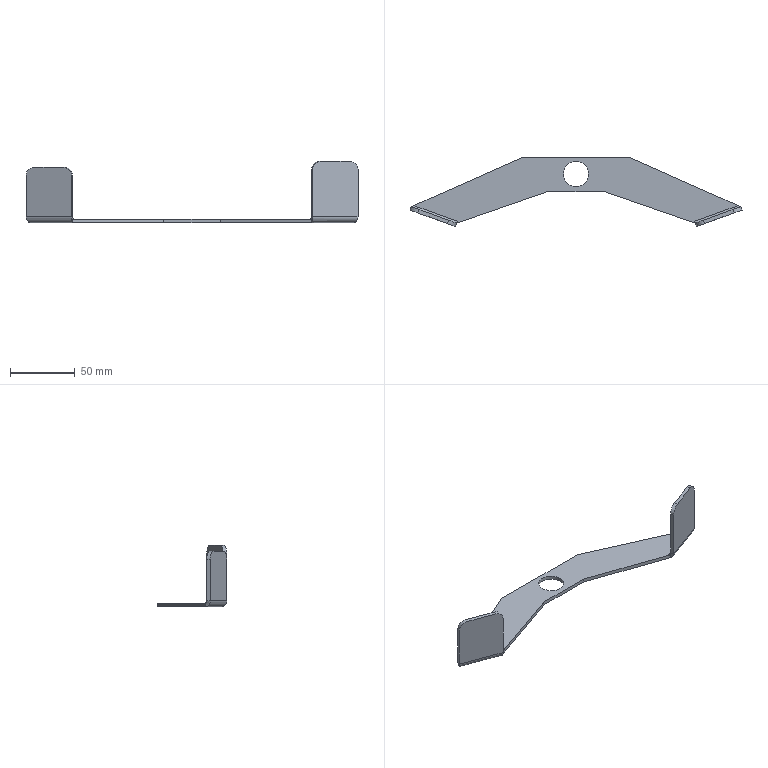Part | NX | features BREP 1 | 1 solid | 36 faces | box 255.894 x 53.402 x 47.219 mm | volume 25837 mm3 | plane 24 | cylinder 10 | spline 2 | commonest cylinder face diameters 12.7 x4 3.175 x2 8.712 x2 19.304 x2
STEP:
#1=CARTESIAN_POINT('',(124.91,13.64,0.));
#2=VERTEX_POINT('',#1);
#3=CARTESIAN_POINT('',(41.275,50.8,0.));
#4=VERTEX_POINT('',#3);
#5=CARTESIAN_POINT('',(124.91,13.64,0.));
#6=DIRECTION('',(-0.9139,0.406,0.));
#7=VECTOR('',#6,1000.);
#8=LINE('',#5,#7);
#9=EDGE_CURVE('',#2,#4,#8,.T.);
#10=ORIENTED_EDGE('',*,*,#9,.T.);
#11=CARTESIAN_POINT('',(-41.275,50.8,0.));
#12=VERTEX_POINT('',#11);
#13=CARTESIAN_POINT('',(41.275,50.8,0.));
#14=DIRECTION('',(-1.,0.,0.));
#15=VECTOR('',#14,1000.);
#16=LINE('',#13,#15);
#17=EDGE_CURVE('',#4,#12,#16,.T.);
#18=ORIENTED_EDGE('',*,*,#17,.T.);
#19=CARTESIAN_POINT('',(-124.91,13.64,0.));
#20=VERTEX_POINT('',#19);
#21=CARTESIAN_POINT('',(-41.275,50.8,0.));
#22=DIRECTION('',(-0.9139,-0.406,0.));
#23=VECTOR('',#22,1000.);
#24=LINE('',#21,#23);
#25=EDGE_CURVE('',#12,#20,#24,.T.);
#26=ORIENTED_EDGE('',*,*,#25,.T.);
#27=CARTESIAN_POINT('',(-91.532,1.492,0.));
#28=VERTEX_POINT('',#27);
#29=CARTESIAN_POINT('',(-124.91,13.64,0.));
#30=DIRECTION('',(0.9397,-0.342,0.));
#31=VECTOR('',#30,1000.);
#32=LINE('',#29,#31);
#33=EDGE_CURVE('',#20,#28,#32,.T.);
#34=ORIENTED_EDGE('',*,*,#33,.T.);
#35=CARTESIAN_POINT('',(-92.075,0.,0.));
#36=VERTEX_POINT('',#35);
#37=CARTESIAN_POINT('',(-91.532,1.492,0.));
#38=DIRECTION('',(-0.342,-0.9397,0.));
#39=VECTOR('',#38,1000.);
#40=LINE('',#37,#39);
#41=EDGE_CURVE('',#28,#36,#40,.T.);
#42=ORIENTED_EDGE('',*,*,#41,.T.);
#43=CARTESIAN_POINT('',(-21.717,24.384,0.));
#44=VERTEX_POINT('',#43);
#45=CARTESIAN_POINT('',(-92.075,0.,0.));
#46=DIRECTION('',(0.9449,0.3275,0.));
#47=VECTOR('',#46,1000.);
#48=LINE('',#45,#47);
#49=EDGE_CURVE('',#36,#44,#48,.T.);
#50=ORIENTED_EDGE('',*,*,#49,.T.);
#51=CARTESIAN_POINT('',(21.717,24.384,0.));
#52=VERTEX_POINT('',#51);
#53=CARTESIAN_POINT('',(-21.717,24.384,0.));
#54=DIRECTION('',(1.,0.,0.));
#55=VECTOR('',#54,1000.);
#56=LINE('',#53,#55);
#57=EDGE_CURVE('',#44,#52,#56,.T.);
#58=ORIENTED_EDGE('',*,*,#57,.T.);
#59=CARTESIAN_POINT('',(92.075,0.,0.));
#60=VERTEX_POINT('',#59);
#61=CARTESIAN_POINT('',(21.717,24.384,0.));
#62=DIRECTION('',(0.9449,-0.3275,0.));
#63=VECTOR('',#62,1000.);
#64=LINE('',#61,#63);
#65=EDGE_CURVE('',#52,#60,#64,.T.);
#66=ORIENTED_EDGE('',*,*,#65,.T.);
#67=CARTESIAN_POINT('',(91.532,1.492,0.));
#68=VERTEX_POINT('',#67);
#69=CARTESIAN_POINT('',(91.532,1.492,0.));
#70=DIRECTION('',(0.342,-0.9397,0.));
#71=VECTOR('',#70,1000.);
#72=LINE('',#69,#71);
#73=EDGE_CURVE('',#68,#60,#72,.T.);
#74=ORIENTED_EDGE('',*,*,#73,.F.);
#75=CARTESIAN_POINT('',(91.532,1.492,0.));
#76=DIRECTION('',(0.9397,0.342,0.));
#77=VECTOR('',#76,1000.);
#78=LINE('',#75,#77);
#79=EDGE_CURVE('',#68,#2,#78,.T.);
#80=ORIENTED_EDGE('',*,*,#79,.T.);
#81=EDGE_LOOP('',(#10,#18,#26,#34,#42,#50,#58,#66,#74,#80));
#82=FACE_BOUND('',#81,.T.);
#83=CARTESIAN_POINT('',(9.652,37.974,0.));
#84=VERTEX_POINT('',#83);
#85=CARTESIAN_POINT('',(-9.652,37.974,0.));
#86=VERTEX_POINT('',#85);
#87=CARTESIAN_POINT('',(0.,37.974,0.));
#88=DIRECTION('',(0.,0.,1.));
#89=DIRECTION('',(1.,0.,0.));
#90=AXIS2_PLACEMENT_3D('',#87,#88,#89);
#91=CIRCLE('',#90,9.652);
#92=EDGE_CURVE('',#84,#86,#91,.T.);
#93=ORIENTED_EDGE('',*,*,#92,.F.);
#94=CARTESIAN_POINT('',(0.,37.974,0.));
#95=DIRECTION('',(0.,0.,1.));
#96=DIRECTION('',(-1.,0.,0.));
#97=AXIS2_PLACEMENT_3D('',#94,#95,#96);
#98=CIRCLE('',#97,9.652);
#99=EDGE_CURVE('',#86,#84,#98,.T.);
#100=ORIENTED_EDGE('',*,*,#99,.F.);
#101=EDGE_LOOP('',(#93,#100));
#102=FACE_BOUND('',#101,.T.);
#103=CARTESIAN_POINT('',(0.,0.,0.));
#104=DIRECTION('',(0.,0.,1.));
#105=DIRECTION('',(1.,0.,0.));
#106=AXIS2_PLACEMENT_3D('',#103,#104,#105);
#107=PLANE('',#106);
#108=ADVANCED_FACE('',(#82,#102),#107,.T.);
#109=CARTESIAN_POINT('',(127.,12.712,1.587));
#110=VERTEX_POINT('',#109);
#111=CARTESIAN_POINT('',(127.,12.712,1.587));
#112=CARTESIAN_POINT('',(126.484,12.524,0.7563));
#113=CARTESIAN_POINT('',(125.71,13.047,0.));
#114=CARTESIAN_POINT('',(124.91,13.64,0.));
#115=B_SPLINE_CURVE_WITH_KNOTS('',3,(#111,#112,#113,#114),.UNSPECIFIED.,.F.,.F.,(4,4),(0.,1.),.UNSPECIFIED.);
#116=EDGE_CURVE('',#110,#2,#115,.T.);
#117=ORIENTED_EDGE('',*,*,#116,.T.);
#118=ORIENTED_EDGE('',*,*,#79,.F.);
#119=CARTESIAN_POINT('',(91.858,0.5973,0.3171));
#120=VERTEX_POINT('',#119);
#121=CARTESIAN_POINT('',(91.532,1.492,1.587));
#122=DIRECTION('',(0.9397,0.342,0.));
#123=DIRECTION('',(0.2051,-0.5635,-0.8003));
#124=AXIS2_PLACEMENT_3D('',#121,#122,#123);
#125=CIRCLE('',#124,1.587);
#126=EDGE_CURVE('',#120,#68,#125,.T.);
#127=ORIENTED_EDGE('',*,*,#126,.F.);
#128=CARTESIAN_POINT('',(92.075,0.,1.587));
#129=VERTEX_POINT('',#128);
#130=CARTESIAN_POINT('',(91.532,1.492,1.587));
#131=DIRECTION('',(0.9397,0.342,0.));
#132=DIRECTION('',(0.342,-0.9397,0.));
#133=AXIS2_PLACEMENT_3D('',#130,#131,#132);
#134=CIRCLE('',#133,1.587);
#135=EDGE_CURVE('',#129,#120,#134,.T.);
#136=ORIENTED_EDGE('',*,*,#135,.F.);
#137=CARTESIAN_POINT('',(92.075,0.,1.587));
#138=DIRECTION('',(0.9397,0.342,0.));
#139=VECTOR('',#138,1000.);
#140=LINE('',#137,#139);
#141=EDGE_CURVE('',#129,#110,#140,.T.);
#142=ORIENTED_EDGE('',*,*,#141,.T.);
#143=EDGE_LOOP('',(#117,#118,#127,#136,#142));
#144=FACE_BOUND('',#143,.T.);
#145=CARTESIAN_POINT('',(91.532,1.492,1.587));
#146=DIRECTION('',(0.9397,0.342,0.));
#147=DIRECTION('',(0.342,-0.9397,0.));
#148=AXIS2_PLACEMENT_3D('',#145,#146,#147);
#149=CYLINDRICAL_SURFACE('',#148,1.587);
#150=ADVANCED_FACE('',(#144),#149,.F.);
#151=ORIENTED_EDGE('',*,*,#141,.F.);
#152=CARTESIAN_POINT('',(92.075,0.,38.1));
#153=VERTEX_POINT('',#152);
#154=CARTESIAN_POINT('',(92.075,0.,38.1));
#155=DIRECTION('',(0.,0.,-1.));
#156=VECTOR('',#155,1000.);
#157=LINE('',#154,#156);
#158=EDGE_CURVE('',#153,#129,#157,.T.);
#159=ORIENTED_EDGE('',*,*,#158,.F.);
#160=CARTESIAN_POINT('',(98.042,2.172,44.45));
#161=VERTEX_POINT('',#160);
#162=CARTESIAN_POINT('',(98.042,2.172,38.1));
#163=DIRECTION('',(0.342,-0.9397,0.));
#164=DIRECTION('',(0.,0.,1.));
#165=AXIS2_PLACEMENT_3D('',#162,#163,#164);
#166=CIRCLE('',#165,6.35);
#167=EDGE_CURVE('',#161,#153,#166,.T.);
#168=ORIENTED_EDGE('',*,*,#167,.F.);
#169=CARTESIAN_POINT('',(121.033,10.54,44.45));
#170=VERTEX_POINT('',#169);
#171=CARTESIAN_POINT('',(121.033,10.54,44.45));
#172=DIRECTION('',(-0.9397,-0.342,0.));
#173=VECTOR('',#172,1000.);
#174=LINE('',#171,#173);
#175=EDGE_CURVE('',#170,#161,#174,.T.);
#176=ORIENTED_EDGE('',*,*,#175,.F.);
#177=CARTESIAN_POINT('',(127.,12.712,38.1));
#178=VERTEX_POINT('',#177);
#179=CARTESIAN_POINT('',(121.033,10.54,38.1));
#180=DIRECTION('',(0.342,-0.9397,0.));
#181=DIRECTION('',(0.9397,0.342,0.));
#182=AXIS2_PLACEMENT_3D('',#179,#180,#181);
#183=CIRCLE('',#182,6.35);
#184=EDGE_CURVE('',#178,#170,#183,.T.);
#185=ORIENTED_EDGE('',*,*,#184,.F.);
#186=CARTESIAN_POINT('',(127.,12.712,1.587));
#187=DIRECTION('',(0.,0.,1.));
#188=VECTOR('',#187,1000.);
#189=LINE('',#186,#188);
#190=EDGE_CURVE('',#110,#178,#189,.T.);
#191=ORIENTED_EDGE('',*,*,#190,.F.);
#192=EDGE_LOOP('',(#151,#159,#168,#176,#185,#191));
#193=FACE_BOUND('',#192,.T.);
#194=CARTESIAN_POINT('',(100.373,3.02,0.));
#195=DIRECTION('',(0.342,-0.9397,0.));
#196=DIRECTION('',(0.,0.,-1.));
#197=AXIS2_PLACEMENT_3D('',#194,#195,#196);
#198=PLANE('',#197);
#199=ADVANCED_FACE('',(#193),#198,.F.);
#200=CARTESIAN_POINT('',(127.947,10.11,38.1));
#201=VERTEX_POINT('',#200);
#202=CARTESIAN_POINT('',(127.,12.712,38.1));
#203=DIRECTION('',(0.342,-0.9397,0.));
#204=VECTOR('',#203,1000.);
#205=LINE('',#202,#204);
#206=EDGE_CURVE('',#178,#201,#205,.T.);
#207=ORIENTED_EDGE('',*,*,#206,.T.);
#208=CARTESIAN_POINT('',(127.947,10.11,1.587));
#209=VERTEX_POINT('',#208);
#210=CARTESIAN_POINT('',(127.947,10.11,1.587));
#211=DIRECTION('',(0.,0.,1.));
#212=VECTOR('',#211,1000.);
#213=LINE('',#210,#212);
#214=EDGE_CURVE('',#209,#201,#213,.T.);
#215=ORIENTED_EDGE('',*,*,#214,.F.);
#216=CARTESIAN_POINT('',(127.,12.712,1.587));
#217=DIRECTION('',(0.342,-0.9397,0.));
#218=VECTOR('',#217,1000.);
#219=LINE('',#216,#218);
#220=EDGE_CURVE('',#110,#209,#219,.T.);
#221=ORIENTED_EDGE('',*,*,#220,.F.);
#222=ORIENTED_EDGE('',*,*,#190,.T.);
#223=EDGE_LOOP('',(#207,#215,#221,#222));
#224=FACE_BOUND('',#223,.T.);
#225=CARTESIAN_POINT('',(127.473,11.411,19.844));
#226=DIRECTION('',(-0.9397,-0.342,0.));
#227=DIRECTION('',(-0.342,0.9397,0.));
#228=AXIS2_PLACEMENT_3D('',#225,#226,#227);
#229=PLANE('',#228);
#230=ADVANCED_FACE('',(#224),#229,.F.);
#231=ORIENTED_EDGE('',*,*,#220,.T.);
#232=CARTESIAN_POINT('',(124.91,13.64,-2.769));
#233=VERTEX_POINT('',#232);
#234=CARTESIAN_POINT('',(124.91,13.64,-2.769));
#235=CARTESIAN_POINT('',(125.558,12.663,-2.769));
#236=CARTESIAN_POINT('',(126.851,10.715,-1.825));
#237=CARTESIAN_POINT('',(127.689,10.016,0.4471));
#238=CARTESIAN_POINT('',(127.947,10.11,1.587));
#239=B_SPLINE_CURVE_WITH_KNOTS('',3,(#234,#235,#236,#237,#238),.UNSPECIFIED.,.F.,.F.,(4,1,4),(0.,0.5,1.),.UNSPECIFIED.);
#240=EDGE_CURVE('',#209,#233,#239,.F.);
#241=ORIENTED_EDGE('',*,*,#240,.T.);
#242=CARTESIAN_POINT('',(124.91,13.64,0.));
#243=DIRECTION('',(0.,0.,-1.));
#244=VECTOR('',#243,1000.);
#245=LINE('',#242,#244);
#246=EDGE_CURVE('',#2,#233,#245,.T.);
#247=ORIENTED_EDGE('',*,*,#246,.F.);
#248=ORIENTED_EDGE('',*,*,#116,.F.);
#249=EDGE_LOOP('',(#231,#241,#247,#248));
#250=FACE_BOUND('',#249,.T.);
#251=CARTESIAN_POINT('',(127.05,13.089,1.8));
#252=CARTESIAN_POINT('',(127.433,12.037,1.989));
#253=CARTESIAN_POINT('',(127.816,10.985,2.179));
#254=CARTESIAN_POINT('',(128.199,9.933,2.369));
#255=CARTESIAN_POINT('',(126.999,13.058,1.729));
#256=CARTESIAN_POINT('',(127.386,11.995,1.857));
#257=CARTESIAN_POINT('',(127.772,10.933,1.984));
#258=CARTESIAN_POINT('',(128.159,9.871,2.111));
#259=CARTESIAN_POINT('',(126.847,12.984,1.526));
#260=CARTESIAN_POINT('',(127.239,11.907,1.47));
#261=CARTESIAN_POINT('',(127.63,10.83,1.415));
#262=CARTESIAN_POINT('',(128.022,9.753,1.36));
#263=CARTESIAN_POINT('',(126.65,12.952,1.289));
#264=CARTESIAN_POINT('',(127.03,11.907,1.021));
#265=CARTESIAN_POINT('',(127.411,10.862,0.7535));
#266=CARTESIAN_POINT('',(127.791,9.816,0.4859));
#267=CARTESIAN_POINT('',(126.412,12.963,1.039));
#268=CARTESIAN_POINT('',(126.764,11.996,0.5485));
#269=CARTESIAN_POINT('',(127.116,11.028,0.05754));
#270=CARTESIAN_POINT('',(127.469,10.06,-0.4334));
#271=CARTESIAN_POINT('',(126.224,12.999,0.8646));
#272=CARTESIAN_POINT('',(126.546,12.114,0.2168));
#273=CARTESIAN_POINT('',(126.868,11.229,-0.431));
#274=CARTESIAN_POINT('',(127.19,10.343,-1.079));
#275=CARTESIAN_POINT('',(125.991,13.076,0.6871));
#276=CARTESIAN_POINT('',(126.267,12.318,-0.1193));
#277=CARTESIAN_POINT('',(126.543,11.56,-0.9257));
#278=CARTESIAN_POINT('',(126.819,10.802,-1.732));
#279=CARTESIAN_POINT('',(125.75,13.177,0.536));
#280=CARTESIAN_POINT('',(125.972,12.568,-0.4062));
#281=CARTESIAN_POINT('',(126.193,11.959,-1.348));
#282=CARTESIAN_POINT('',(126.415,11.351,-2.291));
#283=CARTESIAN_POINT('',(125.536,13.285,0.4378));
#284=CARTESIAN_POINT('',(125.704,12.823,-0.5921));
#285=CARTESIAN_POINT('',(125.872,12.362,-1.622));
#286=CARTESIAN_POINT('',(126.039,11.901,-2.652));
#287=CARTESIAN_POINT('',(125.244,13.444,0.346));
#288=CARTESIAN_POINT('',(125.336,13.193,-0.7664));
#289=CARTESIAN_POINT('',(125.427,12.941,-1.879));
#290=CARTESIAN_POINT('',(125.519,12.69,-2.991));
#291=CARTESIAN_POINT('',(124.979,13.6,0.3082));
#292=CARTESIAN_POINT('',(124.998,13.548,-0.8377));
#293=CARTESIAN_POINT('',(125.017,13.496,-1.984));
#294=CARTESIAN_POINT('',(125.036,13.444,-3.13));
#295=CARTESIAN_POINT('',(124.751,13.734,0.3256));
#296=CARTESIAN_POINT('',(124.708,13.853,-0.8049));
#297=CARTESIAN_POINT('',(124.664,13.973,-1.935));
#298=CARTESIAN_POINT('',(124.621,14.092,-3.066));
#299=CARTESIAN_POINT('',(124.672,13.779,0.3379));
#300=CARTESIAN_POINT('',(124.607,13.958,-0.7818));
#301=CARTESIAN_POINT('',(124.542,14.136,-1.901));
#302=CARTESIAN_POINT('',(124.477,14.315,-3.021));
#303=B_SPLINE_SURFACE_WITH_KNOTS('',3,3,((#251,#252,#253,#254),(#255,#256,#257,#258),(#259,#260,#261,#262),(#263,#264,#265,#266),(#267,#268,#269,#270),(#271,#272,#273,#274),(#275,#276,#277,#278),(#279,#280,#281,#282),(#283,#284,#285,#286),(#287,#288,#289,#290),(#291,#292,#293,#294),(#295,#296,#297,#298),(#299,#300,#301,#302)),.UNSPECIFIED.,.F.,.F.,.F.,(4,1,1,1,1,1,1,1,1,1,4),(4,4),(-0.1069,0.,0.2,0.25,0.4,0.5,0.6,0.75,0.8,1.,1.107),(-0.1154,1.115),.UNSPECIFIED.);
#304=ADVANCED_FACE('',(#250),#303,.F.);
#305=ORIENTED_EDGE('',*,*,#246,.T.);
#306=CARTESIAN_POINT('',(41.275,50.8,-2.769));
#307=VERTEX_POINT('',#306);
#308=CARTESIAN_POINT('',(124.91,13.64,-2.769));
#309=DIRECTION('',(-0.9139,0.406,0.));
#310=VECTOR('',#309,1000.);
#311=LINE('',#308,#310);
#312=EDGE_CURVE('',#233,#307,#311,.T.);
#313=ORIENTED_EDGE('',*,*,#312,.T.);
#314=CARTESIAN_POINT('',(41.275,50.8,0.));
#315=DIRECTION('',(0.,0.,-1.));
#316=VECTOR('',#315,1000.);
#317=LINE('',#314,#316);
#318=EDGE_CURVE('',#4,#307,#317,.T.);
#319=ORIENTED_EDGE('',*,*,#318,.F.);
#320=ORIENTED_EDGE('',*,*,#9,.F.);
#321=EDGE_LOOP('',(#305,#313,#319,#320));
#322=FACE_BOUND('',#321,.T.);
#323=CARTESIAN_POINT('',(84.138,31.756,-1.384));
#324=DIRECTION('',(0.406,0.9139,0.));
#325=DIRECTION('',(0.,0.,-1.));
#326=AXIS2_PLACEMENT_3D('',#323,#324,#325);
#327=PLANE('',#326);
#328=ADVANCED_FACE('',(#322),#327,.T.);
#329=ORIENTED_EDGE('',*,*,#318,.T.);
#330=CARTESIAN_POINT('',(-41.275,50.8,-2.769));
#331=VERTEX_POINT('',#330);
#332=CARTESIAN_POINT('',(41.275,50.8,-2.769));
#333=DIRECTION('',(-1.,0.,0.));
#334=VECTOR('',#333,1000.);
#335=LINE('',#332,#334);
#336=EDGE_CURVE('',#307,#331,#335,.T.);
#337=ORIENTED_EDGE('',*,*,#336,.T.);
#338=CARTESIAN_POINT('',(-41.275,50.8,0.));
#339=DIRECTION('',(0.,0.,-1.));
#340=VECTOR('',#339,1000.);
#341=LINE('',#338,#340);
#342=EDGE_CURVE('',#12,#331,#341,.T.);
#343=ORIENTED_EDGE('',*,*,#342,.F.);
#344=ORIENTED_EDGE('',*,*,#17,.F.);
#345=EDGE_LOOP('',(#329,#337,#343,#344));
#346=FACE_BOUND('',#345,.T.);
#347=CARTESIAN_POINT('',(0.,50.8,-1.384));
#348=DIRECTION('',(0.,1.,0.));
#349=DIRECTION('',(1.,0.,0.));
#350=AXIS2_PLACEMENT_3D('',#347,#348,#349);
#351=PLANE('',#350);
#352=ADVANCED_FACE('',(#346),#351,.T.);
#353=ORIENTED_EDGE('',*,*,#342,.T.);
#354=CARTESIAN_POINT('',(-124.91,13.64,-2.769));
#355=VERTEX_POINT('',#354);
#356=CARTESIAN_POINT('',(-41.275,50.8,-2.769));
#357=DIRECTION('',(-0.9139,-0.406,0.));
#358=VECTOR('',#357,1000.);
#359=LINE('',#356,#358);
#360=EDGE_CURVE('',#331,#355,#359,.T.);
#361=ORIENTED_EDGE('',*,*,#360,.T.);
#362=CARTESIAN_POINT('',(-124.91,13.64,0.));
#363=DIRECTION('',(0.,0.,-1.));
#364=VECTOR('',#363,1000.);
#365=LINE('',#362,#364);
#366=EDGE_CURVE('',#20,#355,#365,.T.);
#367=ORIENTED_EDGE('',*,*,#366,.F.);
#368=ORIENTED_EDGE('',*,*,#25,.F.);
#369=EDGE_LOOP('',(#353,#361,#367,#368));
#370=FACE_BOUND('',#369,.T.);
#371=CARTESIAN_POINT('',(-84.138,31.756,-1.384));
#372=DIRECTION('',(-0.406,0.9139,0.));
#373=DIRECTION('',(0.,0.,1.));
#374=AXIS2_PLACEMENT_3D('',#371,#372,#373);
#375=PLANE('',#374);
#376=ADVANCED_FACE('',(#370),#375,.T.);
#377=ORIENTED_EDGE('',*,*,#366,.T.);
#378=CARTESIAN_POINT('',(-127.947,10.11,1.587));
#379=VERTEX_POINT('',#378);
#380=CARTESIAN_POINT('',(-127.947,10.11,1.587));
#381=CARTESIAN_POINT('',(-127.689,10.016,0.4471));
#382=CARTESIAN_POINT('',(-126.851,10.715,-1.825));
#383=CARTESIAN_POINT('',(-125.558,12.663,-2.769));
#384=CARTESIAN_POINT('',(-124.91,13.64,-2.769));
#385=B_SPLINE_CURVE_WITH_KNOTS('',3,(#380,#381,#382,#383,#384),.UNSPECIFIED.,.F.,.F.,(4,1,4),(0.,0.5,1.),.UNSPECIFIED.);
#386=EDGE_CURVE('',#379,#355,#385,.T.);
#387=ORIENTED_EDGE('',*,*,#386,.F.);
#388=CARTESIAN_POINT('',(-127.,12.712,1.587));
#389=VERTEX_POINT('',#388);
#390=CARTESIAN_POINT('',(-127.,12.712,1.587));
#391=DIRECTION('',(-0.342,-0.9397,0.));
#392=VECTOR('',#391,1000.);
#393=LINE('',#390,#392);
#394=EDGE_CURVE('',#389,#379,#393,.T.);
#395=ORIENTED_EDGE('',*,*,#394,.F.);
#396=CARTESIAN_POINT('',(-124.91,13.64,0.));
#397=CARTESIAN_POINT('',(-125.71,13.047,0.));
#398=CARTESIAN_POINT('',(-126.484,12.524,0.7563));
#399=CARTESIAN_POINT('',(-127.,12.712,1.587));
#400=B_SPLINE_CURVE_WITH_KNOTS('',3,(#396,#397,#398,#399),.UNSPECIFIED.,.F.,.F.,(4,4),(0.,1.),.UNSPECIFIED.);
#401=EDGE_CURVE('',#389,#20,#400,.F.);
#402=ORIENTED_EDGE('',*,*,#401,.T.);
#403=EDGE_LOOP('',(#377,#387,#395,#402));
#404=FACE_BOUND('',#403,.T.);
#405=CARTESIAN_POINT('',(-127.05,13.089,1.8));
#406=CARTESIAN_POINT('',(-127.433,12.037,1.989));
#407=CARTESIAN_POINT('',(-127.816,10.985,2.179));
#408=CARTESIAN_POINT('',(-128.199,9.933,2.369));
#409=CARTESIAN_POINT('',(-126.999,13.058,1.729));
#410=CARTESIAN_POINT('',(-127.386,11.995,1.857));
#411=CARTESIAN_POINT('',(-127.772,10.933,1.984));
#412=CARTESIAN_POINT('',(-128.159,9.871,2.111));
#413=CARTESIAN_POINT('',(-126.847,12.984,1.526));
#414=CARTESIAN_POINT('',(-127.239,11.907,1.47));
#415=CARTESIAN_POINT('',(-127.63,10.83,1.415));
#416=CARTESIAN_POINT('',(-128.022,9.753,1.36));
#417=CARTESIAN_POINT('',(-126.65,12.952,1.289));
#418=CARTESIAN_POINT('',(-127.03,11.907,1.021));
#419=CARTESIAN_POINT('',(-127.411,10.862,0.7535));
#420=CARTESIAN_POINT('',(-127.791,9.816,0.4859));
#421=CARTESIAN_POINT('',(-126.412,12.963,1.039));
#422=CARTESIAN_POINT('',(-126.764,11.996,0.5485));
#423=CARTESIAN_POINT('',(-127.116,11.028,0.05754));
#424=CARTESIAN_POINT('',(-127.469,10.06,-0.4334));
#425=CARTESIAN_POINT('',(-126.224,12.999,0.8646));
#426=CARTESIAN_POINT('',(-126.546,12.114,0.2168));
#427=CARTESIAN_POINT('',(-126.868,11.229,-0.431));
#428=CARTESIAN_POINT('',(-127.19,10.343,-1.079));
#429=CARTESIAN_POINT('',(-125.991,13.076,0.6871));
#430=CARTESIAN_POINT('',(-126.267,12.318,-0.1193));
#431=CARTESIAN_POINT('',(-126.543,11.56,-0.9257));
#432=CARTESIAN_POINT('',(-126.819,10.802,-1.732));
#433=CARTESIAN_POINT('',(-125.75,13.177,0.536));
#434=CARTESIAN_POINT('',(-125.972,12.568,-0.4062));
#435=CARTESIAN_POINT('',(-126.193,11.959,-1.348));
#436=CARTESIAN_POINT('',(-126.415,11.351,-2.291));
#437=CARTESIAN_POINT('',(-125.536,13.285,0.4378));
#438=CARTESIAN_POINT('',(-125.704,12.823,-0.5921));
#439=CARTESIAN_POINT('',(-125.872,12.362,-1.622));
#440=CARTESIAN_POINT('',(-126.039,11.901,-2.652));
#441=CARTESIAN_POINT('',(-125.244,13.444,0.346));
#442=CARTESIAN_POINT('',(-125.336,13.193,-0.7664));
#443=CARTESIAN_POINT('',(-125.427,12.941,-1.879));
#444=CARTESIAN_POINT('',(-125.519,12.69,-2.991));
#445=CARTESIAN_POINT('',(-124.979,13.6,0.3082));
#446=CARTESIAN_POINT('',(-124.998,13.548,-0.8377));
#447=CARTESIAN_POINT('',(-125.017,13.496,-1.984));
#448=CARTESIAN_POINT('',(-125.036,13.444,-3.13));
#449=CARTESIAN_POINT('',(-124.751,13.734,0.3256));
#450=CARTESIAN_POINT('',(-124.708,13.853,-0.8049));
#451=CARTESIAN_POINT('',(-124.664,13.973,-1.935));
#452=CARTESIAN_POINT('',(-124.621,14.092,-3.066));
#453=CARTESIAN_POINT('',(-124.672,13.779,0.3379));
#454=CARTESIAN_POINT('',(-124.607,13.958,-0.7818));
#455=CARTESIAN_POINT('',(-124.542,14.136,-1.901));
#456=CARTESIAN_POINT('',(-124.477,14.315,-3.021));
#457=B_SPLINE_SURFACE_WITH_KNOTS('',3,3,((#405,#406,#407,#408),(#409,#410,#411,#412),(#413,#414,#415,#416),(#417,#418,#419,#420),(#421,#422,#423,#424),(#425,#426,#427,#428),(#429,#430,#431,#432),(#433,#434,#435,#436),(#437,#438,#439,#440),(#441,#442,#443,#444),(#445,#446,#447,#448),(#449,#450,#451,#452),(#453,#454,#455,#456)),.UNSPECIFIED.,.F.,.F.,.F.,(4,1,1,1,1,1,1,1,1,1,4),(4,4),(-0.1069,0.,0.2,0.25,0.4,0.5,0.6,0.75,0.8,1.,1.107),(-0.1154,1.115),.UNSPECIFIED.);
#458=ADVANCED_FACE('',(#404),#457,.T.);
#459=CARTESIAN_POINT('',(-92.075,0.,1.587));
#460=VERTEX_POINT('',#459);
#461=CARTESIAN_POINT('',(-91.858,0.5973,0.3171));
#462=VERTEX_POINT('',#461);
#463=CARTESIAN_POINT('',(-91.532,1.492,1.587));
#464=DIRECTION('',(0.9397,-0.342,0.));
#465=DIRECTION('',(-0.342,-0.9397,0.));
#466=AXIS2_PLACEMENT_3D('',#463,#464,#465);
#467=CIRCLE('',#466,1.587);
#468=EDGE_CURVE('',#460,#462,#467,.T.);
#469=ORIENTED_EDGE('',*,*,#468,.T.);
#470=CARTESIAN_POINT('',(-91.532,1.492,1.587));
#471=DIRECTION('',(0.9397,-0.342,0.));
#472=DIRECTION('',(-0.2051,-0.5635,-0.8003));
#473=AXIS2_PLACEMENT_3D('',#470,#471,#472);
#474=CIRCLE('',#473,1.587);
#475=EDGE_CURVE('',#462,#28,#474,.T.);
#476=ORIENTED_EDGE('',*,*,#475,.T.);
#477=ORIENTED_EDGE('',*,*,#33,.F.);
#478=ORIENTED_EDGE('',*,*,#401,.F.);
#479=CARTESIAN_POINT('',(-127.,12.712,1.587));
#480=DIRECTION('',(0.9397,-0.342,0.));
#481=VECTOR('',#480,1000.);
#482=LINE('',#479,#481);
#483=EDGE_CURVE('',#389,#460,#482,.T.);
#484=ORIENTED_EDGE('',*,*,#483,.T.);
#485=EDGE_LOOP('',(#469,#476,#477,#478,#484));
#486=FACE_BOUND('',#485,.T.);
#487=CARTESIAN_POINT('',(-126.457,14.203,1.587));
#488=DIRECTION('',(0.9397,-0.342,0.));
#489=DIRECTION('',(-0.342,-0.9397,0.));
#490=AXIS2_PLACEMENT_3D('',#487,#488,#489);
#491=CYLINDRICAL_SURFACE('',#490,1.587);
#492=ADVANCED_FACE('',(#486),#491,.F.);
#493=ORIENTED_EDGE('',*,*,#483,.F.);
#494=CARTESIAN_POINT('',(-127.,12.712,33.528));
#495=VERTEX_POINT('',#494);
#496=CARTESIAN_POINT('',(-127.,12.712,33.528));
#497=DIRECTION('',(0.,0.,-1.));
#498=VECTOR('',#497,1000.);
#499=LINE('',#496,#498);
#500=EDGE_CURVE('',#495,#389,#499,.T.);
#501=ORIENTED_EDGE('',*,*,#500,.F.);
#502=CARTESIAN_POINT('',(-121.033,10.54,39.878));
#503=VERTEX_POINT('',#502);
#504=CARTESIAN_POINT('',(-121.033,10.54,33.528));
#505=DIRECTION('',(-0.342,-0.9397,0.));
#506=DIRECTION('',(0.,0.,1.));
#507=AXIS2_PLACEMENT_3D('',#504,#505,#506);
#508=CIRCLE('',#507,6.35);
#509=EDGE_CURVE('',#503,#495,#508,.T.);
#510=ORIENTED_EDGE('',*,*,#509,.F.);
#511=CARTESIAN_POINT('',(-98.042,2.172,39.878));
#512=VERTEX_POINT('',#511);
#513=CARTESIAN_POINT('',(-98.042,2.172,39.878));
#514=DIRECTION('',(-0.9397,0.342,0.));
#515=VECTOR('',#514,1000.);
#516=LINE('',#513,#515);
#517=EDGE_CURVE('',#512,#503,#516,.T.);
#518=ORIENTED_EDGE('',*,*,#517,.F.);
#519=CARTESIAN_POINT('',(-92.075,0.,33.528));
#520=VERTEX_POINT('',#519);
#521=CARTESIAN_POINT('',(-98.042,2.172,33.528));
#522=DIRECTION('',(-0.342,-0.9397,0.));
#523=DIRECTION('',(0.9397,-0.342,0.));
#524=AXIS2_PLACEMENT_3D('',#521,#522,#523);
#525=CIRCLE('',#524,6.35);
#526=EDGE_CURVE('',#520,#512,#525,.T.);
#527=ORIENTED_EDGE('',*,*,#526,.F.);
#528=CARTESIAN_POINT('',(-92.075,0.,1.587));
#529=DIRECTION('',(0.,0.,1.));
#530=VECTOR('',#529,1000.);
#531=LINE('',#528,#530);
#532=EDGE_CURVE('',#460,#520,#531,.T.);
#533=ORIENTED_EDGE('',*,*,#532,.F.);
#534=EDGE_LOOP('',(#493,#501,#510,#518,#527,#533));
#535=FACE_BOUND('',#534,.T.);
#536=CARTESIAN_POINT('',(-118.702,9.691,0.));
#537=DIRECTION('',(-0.342,-0.9397,0.));
#538=DIRECTION('',(-0.9397,0.342,0.));
#539=AXIS2_PLACEMENT_3D('',#536,#537,#538);
#540=PLANE('',#539);
#541=ADVANCED_FACE('',(#535),#540,.F.);
#542=CARTESIAN_POINT('',(-93.022,-2.602,33.528));
#543=VERTEX_POINT('',#542);
#544=CARTESIAN_POINT('',(-92.075,0.,33.528));
#545=DIRECTION('',(-0.342,-0.9397,0.));
#546=VECTOR('',#545,1000.);
#547=LINE('',#544,#546);
#548=EDGE_CURVE('',#520,#543,#547,.T.);
#549=ORIENTED_EDGE('',*,*,#548,.T.);
#550=CARTESIAN_POINT('',(-93.022,-2.602,1.587));
#551=VERTEX_POINT('',#550);
#552=CARTESIAN_POINT('',(-93.022,-2.602,1.587));
#553=DIRECTION('',(0.,0.,1.));
#554=VECTOR('',#553,1000.);
#555=LINE('',#552,#554);
#556=EDGE_CURVE('',#551,#543,#555,.T.);
#557=ORIENTED_EDGE('',*,*,#556,.F.);
#558=CARTESIAN_POINT('',(-92.075,0.,1.587));
#559=DIRECTION('',(-0.342,-0.9397,0.));
#560=VECTOR('',#559,1000.);
#561=LINE('',#558,#560);
#562=EDGE_CURVE('',#460,#551,#561,.T.);
#563=ORIENTED_EDGE('',*,*,#562,.F.);
#564=ORIENTED_EDGE('',*,*,#532,.T.);
#565=EDGE_LOOP('',(#549,#557,#563,#564));
#566=FACE_BOUND('',#565,.T.);
#567=CARTESIAN_POINT('',(-92.548,-1.301,17.558));
#568=DIRECTION('',(-0.9397,0.342,0.));
#569=DIRECTION('',(0.,0.,1.));
#570=AXIS2_PLACEMENT_3D('',#567,#568,#569);
#571=PLANE('',#570);
#572=ADVANCED_FACE('',(#566),#571,.F.);
#573=ORIENTED_EDGE('',*,*,#562,.T.);
#574=CARTESIAN_POINT('',(-92.425,-0.9627,-1.899));
#575=VERTEX_POINT('',#574);
#576=CARTESIAN_POINT('',(-91.532,1.492,1.587));
#577=DIRECTION('',(0.9397,-0.342,0.));
#578=DIRECTION('',(-0.342,-0.9397,0.));
#579=AXIS2_PLACEMENT_3D('',#576,#577,#578);
#580=CIRCLE('',#579,4.356);
#581=EDGE_CURVE('',#551,#575,#580,.T.);
#582=ORIENTED_EDGE('',*,*,#581,.T.);
#583=CARTESIAN_POINT('',(-91.858,0.5973,0.3171));
#584=DIRECTION('',(-0.2051,-0.5635,-0.8003));
#585=VECTOR('',#584,1000.);
#586=LINE('',#583,#585);
#587=EDGE_CURVE('',#462,#575,#586,.T.);
#588=ORIENTED_EDGE('',*,*,#587,.F.);
#589=ORIENTED_EDGE('',*,*,#468,.F.);
#590=EDGE_LOOP('',(#573,#582,#588,#589));
#591=FACE_BOUND('',#590,.T.);
#592=CARTESIAN_POINT('',(-92.441,-1.006,0.2578));
#593=DIRECTION('',(0.9397,-0.342,0.));
#594=DIRECTION('',(0.,0.,-1.));
#595=AXIS2_PLACEMENT_3D('',#592,#593,#594);
#596=PLANE('',#595);
#597=ADVANCED_FACE('',(#591),#596,.T.);
#598=ORIENTED_EDGE('',*,*,#587,.T.);
#599=CARTESIAN_POINT('',(-91.532,1.492,-2.769));
#600=VERTEX_POINT('',#599);
#601=CARTESIAN_POINT('',(-91.532,1.492,1.587));
#602=DIRECTION('',(0.9397,-0.342,0.));
#603=DIRECTION('',(-0.2051,-0.5635,-0.8003));
#604=AXIS2_PLACEMENT_3D('',#601,#602,#603);
#605=CIRCLE('',#604,4.356);
#606=EDGE_CURVE('',#575,#600,#605,.T.);
#607=ORIENTED_EDGE('',*,*,#606,.T.);
#608=CARTESIAN_POINT('',(-91.532,1.492,0.));
#609=DIRECTION('',(0.,0.,-1.));
#610=VECTOR('',#609,1000.);
#611=LINE('',#608,#610);
#612=EDGE_CURVE('',#28,#600,#611,.T.);
#613=ORIENTED_EDGE('',*,*,#612,.F.);
#614=ORIENTED_EDGE('',*,*,#475,.F.);
#615=EDGE_LOOP('',(#598,#607,#613,#614));
#616=FACE_BOUND('',#615,.T.);
#617=CARTESIAN_POINT('',(-91.853,0.6093,-1.232));
#618=DIRECTION('',(0.9397,-0.342,0.));
#619=DIRECTION('',(0.,0.,-1.));
#620=AXIS2_PLACEMENT_3D('',#617,#618,#619);
#621=PLANE('',#620);
#622=ADVANCED_FACE('',(#616),#621,.T.);
#623=ORIENTED_EDGE('',*,*,#612,.T.);
#624=CARTESIAN_POINT('',(-92.075,0.,-2.769));
#625=VERTEX_POINT('',#624);
#626=CARTESIAN_POINT('',(-91.532,1.492,-2.769));
#627=DIRECTION('',(-0.342,-0.9397,0.));
#628=VECTOR('',#627,1000.);
#629=LINE('',#626,#628);
#630=EDGE_CURVE('',#600,#625,#629,.T.);
#631=ORIENTED_EDGE('',*,*,#630,.T.);
#632=CARTESIAN_POINT('',(-92.075,0.,0.));
#633=DIRECTION('',(0.,0.,-1.));
#634=VECTOR('',#633,1000.);
#635=LINE('',#632,#634);
#636=EDGE_CURVE('',#36,#625,#635,.T.);
#637=ORIENTED_EDGE('',*,*,#636,.F.);
#638=ORIENTED_EDGE('',*,*,#41,.F.);
#639=EDGE_LOOP('',(#623,#631,#637,#638));
#640=FACE_BOUND('',#639,.T.);
#641=CARTESIAN_POINT('',(-91.804,0.7459,-1.384));
#642=DIRECTION('',(-0.9397,0.342,0.));
#643=DIRECTION('',(0.,0.,1.));
#644=AXIS2_PLACEMENT_3D('',#641,#642,#643);
#645=PLANE('',#644);
#646=ADVANCED_FACE('',(#640),#645,.T.);
#647=ORIENTED_EDGE('',*,*,#636,.T.);
#648=CARTESIAN_POINT('',(-21.717,24.384,-2.769));
#649=VERTEX_POINT('',#648);
#650=CARTESIAN_POINT('',(-92.075,0.,-2.769));
#651=DIRECTION('',(0.9449,0.3275,0.));
#652=VECTOR('',#651,1000.);
#653=LINE('',#650,#652);
#654=EDGE_CURVE('',#625,#649,#653,.T.);
#655=ORIENTED_EDGE('',*,*,#654,.T.);
#656=CARTESIAN_POINT('',(-21.717,24.384,0.));
#657=DIRECTION('',(0.,0.,-1.));
#658=VECTOR('',#657,1000.);
#659=LINE('',#656,#658);
#660=EDGE_CURVE('',#44,#649,#659,.T.);
#661=ORIENTED_EDGE('',*,*,#660,.F.);
#662=ORIENTED_EDGE('',*,*,#49,.F.);
#663=EDGE_LOOP('',(#647,#655,#661,#662));
#664=FACE_BOUND('',#663,.T.);
#665=CARTESIAN_POINT('',(-56.896,12.192,-1.384));
#666=DIRECTION('',(0.3275,-0.9449,0.));
#667=DIRECTION('',(0.,0.,-1.));
#668=AXIS2_PLACEMENT_3D('',#665,#666,#667);
#669=PLANE('',#668);
#670=ADVANCED_FACE('',(#664),#669,.T.);
#671=ORIENTED_EDGE('',*,*,#660,.T.);
#672=CARTESIAN_POINT('',(21.717,24.384,-2.769));
#673=VERTEX_POINT('',#672);
#674=CARTESIAN_POINT('',(-21.717,24.384,-2.769));
#675=DIRECTION('',(1.,0.,0.));
#676=VECTOR('',#675,1000.);
#677=LINE('',#674,#676);
#678=EDGE_CURVE('',#649,#673,#677,.T.);
#679=ORIENTED_EDGE('',*,*,#678,.T.);
#680=CARTESIAN_POINT('',(21.717,24.384,0.));
#681=DIRECTION('',(0.,0.,-1.));
#682=VECTOR('',#681,1000.);
#683=LINE('',#680,#682);
#684=EDGE_CURVE('',#52,#673,#683,.T.);
#685=ORIENTED_EDGE('',*,*,#684,.F.);
#686=ORIENTED_EDGE('',*,*,#57,.F.);
#687=EDGE_LOOP('',(#671,#679,#685,#686));
#688=FACE_BOUND('',#687,.T.);
#689=CARTESIAN_POINT('',(0.,24.384,-1.384));
#690=DIRECTION('',(0.,-1.,0.));
#691=DIRECTION('',(0.,0.,-1.));
#692=AXIS2_PLACEMENT_3D('',#689,#690,#691);
#693=PLANE('',#692);
#694=ADVANCED_FACE('',(#688),#693,.T.);
#695=ORIENTED_EDGE('',*,*,#684,.T.);
#696=CARTESIAN_POINT('',(92.075,0.,-2.769));
#697=VERTEX_POINT('',#696);
#698=CARTESIAN_POINT('',(21.717,24.384,-2.769));
#699=DIRECTION('',(0.9449,-0.3275,0.));
#700=VECTOR('',#699,1000.);
#701=LINE('',#698,#700);
#702=EDGE_CURVE('',#673,#697,#701,.T.);
#703=ORIENTED_EDGE('',*,*,#702,.T.);
#704=CARTESIAN_POINT('',(92.075,0.,0.));
#705=DIRECTION('',(0.,0.,-1.));
#706=VECTOR('',#705,1000.);
#707=LINE('',#704,#706);
#708=EDGE_CURVE('',#60,#697,#707,.T.);
#709=ORIENTED_EDGE('',*,*,#708,.F.);
#710=ORIENTED_EDGE('',*,*,#65,.F.);
#711=EDGE_LOOP('',(#695,#703,#709,#710));
#712=FACE_BOUND('',#711,.T.);
#713=CARTESIAN_POINT('',(56.896,12.192,-1.384));
#714=DIRECTION('',(-0.3275,-0.9449,0.));
#715=DIRECTION('',(-0.9449,0.3275,0.));
#716=AXIS2_PLACEMENT_3D('',#713,#714,#715);
#717=PLANE('',#716);
#718=ADVANCED_FACE('',(#712),#717,.T.);
#719=ORIENTED_EDGE('',*,*,#708,.T.);
#720=CARTESIAN_POINT('',(91.532,1.492,-2.769));
#721=VERTEX_POINT('',#720);
#722=CARTESIAN_POINT('',(91.532,1.492,-2.769));
#723=DIRECTION('',(0.342,-0.9397,0.));
#724=VECTOR('',#723,1000.);
#725=LINE('',#722,#724);
#726=EDGE_CURVE('',#721,#697,#725,.T.);
#727=ORIENTED_EDGE('',*,*,#726,.F.);
#728=CARTESIAN_POINT('',(91.532,1.492,0.));
#729=DIRECTION('',(0.,0.,-1.));
#730=VECTOR('',#729,1000.);
#731=LINE('',#728,#730);
#732=EDGE_CURVE('',#68,#721,#731,.T.);
#733=ORIENTED_EDGE('',*,*,#732,.F.);
#734=ORIENTED_EDGE('',*,*,#73,.T.);
#735=EDGE_LOOP('',(#719,#727,#733,#734));
#736=FACE_BOUND('',#735,.T.);
#737=CARTESIAN_POINT('',(91.804,0.7459,-1.384));
#738=DIRECTION('',(-0.9397,-0.342,0.));
#739=DIRECTION('',(-0.342,0.9397,0.));
#740=AXIS2_PLACEMENT_3D('',#737,#738,#739);
#741=PLANE('',#740);
#742=ADVANCED_FACE('',(#736),#741,.F.);
#743=ORIENTED_EDGE('',*,*,#732,.T.);
#744=CARTESIAN_POINT('',(92.425,-0.9627,-1.899));
#745=VERTEX_POINT('',#744);
#746=CARTESIAN_POINT('',(91.532,1.492,1.587));
#747=DIRECTION('',(0.9397,0.342,0.));
#748=DIRECTION('',(0.2051,-0.5635,-0.8003));
#749=AXIS2_PLACEMENT_3D('',#746,#747,#748);
#750=CIRCLE('',#749,4.356);
#751=EDGE_CURVE('',#745,#721,#750,.T.);
#752=ORIENTED_EDGE('',*,*,#751,.F.);
#753=CARTESIAN_POINT('',(91.858,0.5973,0.3171));
#754=DIRECTION('',(0.2051,-0.5635,-0.8003));
#755=VECTOR('',#754,1000.);
#756=LINE('',#753,#755);
#757=EDGE_CURVE('',#120,#745,#756,.T.);
#758=ORIENTED_EDGE('',*,*,#757,.F.);
#759=ORIENTED_EDGE('',*,*,#126,.T.);
#760=EDGE_LOOP('',(#743,#752,#758,#759));
#761=FACE_BOUND('',#760,.T.);
#762=CARTESIAN_POINT('',(91.853,0.6093,-1.232));
#763=DIRECTION('',(0.9397,0.342,0.));
#764=DIRECTION('',(0.,0.,-1.));
#765=AXIS2_PLACEMENT_3D('',#762,#763,#764);
#766=PLANE('',#765);
#767=ADVANCED_FACE('',(#761),#766,.F.);
#768=ORIENTED_EDGE('',*,*,#757,.T.);
#769=CARTESIAN_POINT('',(93.022,-2.602,1.587));
#770=VERTEX_POINT('',#769);
#771=CARTESIAN_POINT('',(91.532,1.492,1.587));
#772=DIRECTION('',(0.9397,0.342,0.));
#773=DIRECTION('',(0.342,-0.9397,0.));
#774=AXIS2_PLACEMENT_3D('',#771,#772,#773);
#775=CIRCLE('',#774,4.356);
#776=EDGE_CURVE('',#770,#745,#775,.T.);
#777=ORIENTED_EDGE('',*,*,#776,.F.);
#778=CARTESIAN_POINT('',(92.075,0.,1.587));
#779=DIRECTION('',(0.342,-0.9397,0.));
#780=VECTOR('',#779,1000.);
#781=LINE('',#778,#780);
#782=EDGE_CURVE('',#129,#770,#781,.T.);
#783=ORIENTED_EDGE('',*,*,#782,.F.);
#784=ORIENTED_EDGE('',*,*,#135,.T.);
#785=EDGE_LOOP('',(#768,#777,#783,#784));
#786=FACE_BOUND('',#785,.T.);
#787=CARTESIAN_POINT('',(92.441,-1.006,0.2578));
#788=DIRECTION('',(0.9397,0.342,0.));
#789=DIRECTION('',(0.,0.,-1.));
#790=AXIS2_PLACEMENT_3D('',#787,#788,#789);
#791=PLANE('',#790);
#792=ADVANCED_FACE('',(#786),#791,.F.);
#793=ORIENTED_EDGE('',*,*,#782,.T.);
#794=CARTESIAN_POINT('',(93.022,-2.602,38.1));
#795=VERTEX_POINT('',#794);
#796=CARTESIAN_POINT('',(93.022,-2.602,38.1));
#797=DIRECTION('',(0.,0.,-1.));
#798=VECTOR('',#797,1000.);
#799=LINE('',#796,#798);
#800=EDGE_CURVE('',#795,#770,#799,.T.);
#801=ORIENTED_EDGE('',*,*,#800,.F.);
#802=CARTESIAN_POINT('',(92.075,0.,38.1));
#803=DIRECTION('',(0.342,-0.9397,0.));
#804=VECTOR('',#803,1000.);
#805=LINE('',#802,#804);
#806=EDGE_CURVE('',#153,#795,#805,.T.);
#807=ORIENTED_EDGE('',*,*,#806,.F.);
#808=ORIENTED_EDGE('',*,*,#158,.T.);
#809=EDGE_LOOP('',(#793,#801,#807,#808));
#810=FACE_BOUND('',#809,.T.);
#811=CARTESIAN_POINT('',(92.548,-1.301,19.844));
#812=DIRECTION('',(0.9397,0.342,0.));
#813=DIRECTION('',(0.,0.,-1.));
#814=AXIS2_PLACEMENT_3D('',#811,#812,#813);
#815=PLANE('',#814);
#816=ADVANCED_FACE('',(#810),#815,.F.);
#817=ORIENTED_EDGE('',*,*,#806,.T.);
#818=CARTESIAN_POINT('',(98.989,-0.4298,44.45));
#819=VERTEX_POINT('',#818);
#820=CARTESIAN_POINT('',(98.989,-0.4298,38.1));
#821=DIRECTION('',(0.342,-0.9397,0.));
#822=DIRECTION('',(0.,0.,1.));
#823=AXIS2_PLACEMENT_3D('',#820,#821,#822);
#824=CIRCLE('',#823,6.35);
#825=EDGE_CURVE('',#819,#795,#824,.T.);
#826=ORIENTED_EDGE('',*,*,#825,.F.);
#827=CARTESIAN_POINT('',(98.042,2.172,44.45));
#828=DIRECTION('',(0.342,-0.9397,0.));
#829=VECTOR('',#828,1000.);
#830=LINE('',#827,#829);
#831=EDGE_CURVE('',#161,#819,#830,.T.);
#832=ORIENTED_EDGE('',*,*,#831,.F.);
#833=ORIENTED_EDGE('',*,*,#167,.T.);
#834=EDGE_LOOP('',(#817,#826,#832,#833));
#835=FACE_BOUND('',#834,.T.);
#836=CARTESIAN_POINT('',(98.516,0.871,38.1));
#837=DIRECTION('',(0.342,-0.9397,0.));
#838=DIRECTION('',(0.,0.,1.));
#839=AXIS2_PLACEMENT_3D('',#836,#837,#838);
#840=CYLINDRICAL_SURFACE('',#839,6.35);
#841=ADVANCED_FACE('',(#835),#840,.T.);
#842=ORIENTED_EDGE('',*,*,#831,.T.);
#843=CARTESIAN_POINT('',(121.98,7.938,44.45));
#844=VERTEX_POINT('',#843);
#845=CARTESIAN_POINT('',(121.98,7.938,44.45));
#846=DIRECTION('',(-0.9397,-0.342,0.));
#847=VECTOR('',#846,1000.);
#848=LINE('',#845,#847);
#849=EDGE_CURVE('',#844,#819,#848,.T.);
#850=ORIENTED_EDGE('',*,*,#849,.F.);
#851=CARTESIAN_POINT('',(121.033,10.54,44.45));
#852=DIRECTION('',(0.342,-0.9397,0.));
#853=VECTOR('',#852,1000.);
#854=LINE('',#851,#853);
#855=EDGE_CURVE('',#170,#844,#854,.T.);
#856=ORIENTED_EDGE('',*,*,#855,.F.);
#857=ORIENTED_EDGE('',*,*,#175,.T.);
#858=EDGE_LOOP('',(#842,#850,#856,#857));
#859=FACE_BOUND('',#858,.T.);
#860=CARTESIAN_POINT('',(110.011,5.055,44.45));
#861=DIRECTION('',(0.,0.,-1.));
#862=DIRECTION('',(0.,-1.,0.));
#863=AXIS2_PLACEMENT_3D('',#860,#861,#862);
#864=PLANE('',#863);
#865=ADVANCED_FACE('',(#859),#864,.F.);
#866=ORIENTED_EDGE('',*,*,#855,.T.);
#867=CARTESIAN_POINT('',(121.98,7.938,38.1));
#868=DIRECTION('',(0.342,-0.9397,0.));
#869=DIRECTION('',(0.9397,0.342,0.));
#870=AXIS2_PLACEMENT_3D('',#867,#868,#869);
#871=CIRCLE('',#870,6.35);
#872=EDGE_CURVE('',#201,#844,#871,.T.);
#873=ORIENTED_EDGE('',*,*,#872,.F.);
#874=ORIENTED_EDGE('',*,*,#206,.F.);
#875=ORIENTED_EDGE('',*,*,#184,.T.);
#876=EDGE_LOOP('',(#866,#873,#874,#875));
#877=FACE_BOUND('',#876,.T.);
#878=CARTESIAN_POINT('',(121.506,9.239,38.1));
#879=DIRECTION('',(0.342,-0.9397,0.));
#880=DIRECTION('',(0.9397,0.342,0.));
#881=AXIS2_PLACEMENT_3D('',#878,#879,#880);
#882=CYLINDRICAL_SURFACE('',#881,6.35);
#883=ADVANCED_FACE('',(#877),#882,.T.);
#884=ORIENTED_EDGE('',*,*,#872,.T.);
#885=ORIENTED_EDGE('',*,*,#849,.T.);
#886=ORIENTED_EDGE('',*,*,#825,.T.);
#887=ORIENTED_EDGE('',*,*,#800,.T.);
#888=CARTESIAN_POINT('',(93.022,-2.602,1.587));
#889=DIRECTION('',(0.9397,0.342,0.));
#890=VECTOR('',#889,1000.);
#891=LINE('',#888,#890);
#892=EDGE_CURVE('',#770,#209,#891,.T.);
#893=ORIENTED_EDGE('',*,*,#892,.T.);
#894=ORIENTED_EDGE('',*,*,#214,.T.);
#895=EDGE_LOOP('',(#884,#885,#886,#887,#893,#894));
#896=FACE_BOUND('',#895,.T.);
#897=CARTESIAN_POINT('',(101.32,0.4187,0.));
#898=DIRECTION('',(0.342,-0.9397,0.));
#899=DIRECTION('',(0.,0.,-1.));
#900=AXIS2_PLACEMENT_3D('',#897,#898,#899);
#901=PLANE('',#900);
#902=ADVANCED_FACE('',(#896),#901,.T.);
#903=ORIENTED_EDGE('',*,*,#776,.T.);
#904=ORIENTED_EDGE('',*,*,#751,.T.);
#905=CARTESIAN_POINT('',(91.532,1.492,-2.769));
#906=DIRECTION('',(0.9397,0.342,0.));
#907=VECTOR('',#906,1000.);
#908=LINE('',#905,#907);
#909=EDGE_CURVE('',#721,#233,#908,.T.);
#910=ORIENTED_EDGE('',*,*,#909,.T.);
#911=ORIENTED_EDGE('',*,*,#240,.F.);
#912=ORIENTED_EDGE('',*,*,#892,.F.);
#913=EDGE_LOOP('',(#903,#904,#910,#911,#912));
#914=FACE_BOUND('',#913,.T.);
#915=CARTESIAN_POINT('',(91.532,1.492,1.587));
#916=DIRECTION('',(0.9397,0.342,0.));
#917=DIRECTION('',(0.342,-0.9397,0.));
#918=AXIS2_PLACEMENT_3D('',#915,#916,#917);
#919=CYLINDRICAL_SURFACE('',#918,4.356);
#920=ADVANCED_FACE('',(#914),#919,.T.);
#921=ORIENTED_EDGE('',*,*,#726,.T.);
#922=ORIENTED_EDGE('',*,*,#702,.F.);
#923=ORIENTED_EDGE('',*,*,#678,.F.);
#924=ORIENTED_EDGE('',*,*,#654,.F.);
#925=ORIENTED_EDGE('',*,*,#630,.F.);
#926=CARTESIAN_POINT('',(-124.91,13.64,-2.769));
#927=DIRECTION('',(0.9397,-0.342,0.));
#928=VECTOR('',#927,1000.);
#929=LINE('',#926,#928);
#930=EDGE_CURVE('',#355,#600,#929,.T.);
#931=ORIENTED_EDGE('',*,*,#930,.F.);
#932=ORIENTED_EDGE('',*,*,#360,.F.);
#933=ORIENTED_EDGE('',*,*,#336,.F.);
#934=ORIENTED_EDGE('',*,*,#312,.F.);
#935=ORIENTED_EDGE('',*,*,#909,.F.);
#936=EDGE_LOOP('',(#921,#922,#923,#924,#925,#931,#932,#933,#934,#935));
#937=FACE_BOUND('',#936,.T.);
#938=CARTESIAN_POINT('',(9.652,37.974,-2.769));
#939=VERTEX_POINT('',#938);
#940=CARTESIAN_POINT('',(-9.652,37.974,-2.769));
#941=VERTEX_POINT('',#940);
#942=CARTESIAN_POINT('',(0.,37.974,-2.769));
#943=DIRECTION('',(0.,0.,1.));
#944=DIRECTION('',(1.,0.,0.));
#945=AXIS2_PLACEMENT_3D('',#942,#943,#944);
#946=CIRCLE('',#945,9.652);
#947=EDGE_CURVE('',#939,#941,#946,.T.);
#948=ORIENTED_EDGE('',*,*,#947,.T.);
#949=CARTESIAN_POINT('',(0.,37.974,-2.769));
#950=DIRECTION('',(0.,0.,1.));
#951=DIRECTION('',(-1.,0.,0.));
#952=AXIS2_PLACEMENT_3D('',#949,#950,#951);
#953=CIRCLE('',#952,9.652);
#954=EDGE_CURVE('',#941,#939,#953,.T.);
#955=ORIENTED_EDGE('',*,*,#954,.T.);
#956=EDGE_LOOP('',(#948,#955));
#957=FACE_BOUND('',#956,.T.);
#958=CARTESIAN_POINT('',(0.,0.,-2.769));
#959=DIRECTION('',(0.,0.,1.));
#960=DIRECTION('',(1.,0.,0.));
#961=AXIS2_PLACEMENT_3D('',#958,#959,#960);
#962=PLANE('',#961);
#963=ADVANCED_FACE('',(#937,#957),#962,.F.);
#964=ORIENTED_EDGE('',*,*,#386,.T.);
#965=ORIENTED_EDGE('',*,*,#930,.T.);
#966=ORIENTED_EDGE('',*,*,#606,.F.);
#967=ORIENTED_EDGE('',*,*,#581,.F.);
#968=CARTESIAN_POINT('',(-127.947,10.11,1.587));
#969=DIRECTION('',(0.9397,-0.342,0.));
#970=VECTOR('',#969,1000.);
#971=LINE('',#968,#970);
#972=EDGE_CURVE('',#379,#551,#971,.T.);
#973=ORIENTED_EDGE('',*,*,#972,.F.);
#974=EDGE_LOOP('',(#964,#965,#966,#967,#973));
#975=FACE_BOUND('',#974,.T.);
#976=CARTESIAN_POINT('',(-126.457,14.203,1.587));
#977=DIRECTION('',(0.9397,-0.342,0.));
#978=DIRECTION('',(-0.342,-0.9397,0.));
#979=AXIS2_PLACEMENT_3D('',#976,#977,#978);
#980=CYLINDRICAL_SURFACE('',#979,4.356);
#981=ADVANCED_FACE('',(#975),#980,.T.);
#982=CARTESIAN_POINT('',(-98.989,-0.4298,39.878));
#983=VERTEX_POINT('',#982);
#984=CARTESIAN_POINT('',(-98.989,-0.4298,33.528));
#985=DIRECTION('',(-0.342,-0.9397,0.));
#986=DIRECTION('',(0.9397,-0.342,0.));
#987=AXIS2_PLACEMENT_3D('',#984,#985,#986);
#988=CIRCLE('',#987,6.35);
#989=EDGE_CURVE('',#543,#983,#988,.T.);
#990=ORIENTED_EDGE('',*,*,#989,.T.);
#991=CARTESIAN_POINT('',(-121.98,7.938,39.878));
#992=VERTEX_POINT('',#991);
#993=CARTESIAN_POINT('',(-98.989,-0.4298,39.878));
#994=DIRECTION('',(-0.9397,0.342,0.));
#995=VECTOR('',#994,1000.);
#996=LINE('',#993,#995);
#997=EDGE_CURVE('',#983,#992,#996,.T.);
#998=ORIENTED_EDGE('',*,*,#997,.T.);
#999=CARTESIAN_POINT('',(-127.947,10.11,33.528));
#1000=VERTEX_POINT('',#999);
#1001=CARTESIAN_POINT('',(-121.98,7.938,33.528));
#1002=DIRECTION('',(-0.342,-0.9397,0.));
#1003=DIRECTION('',(0.,0.,1.));
#1004=AXIS2_PLACEMENT_3D('',#1001,#1002,#1003);
#1005=CIRCLE('',#1004,6.35);
#1006=EDGE_CURVE('',#992,#1000,#1005,.T.);
#1007=ORIENTED_EDGE('',*,*,#1006,.T.);
#1008=CARTESIAN_POINT('',(-127.947,10.11,33.528));
#1009=DIRECTION('',(0.,0.,-1.));
#1010=VECTOR('',#1009,1000.);
#1011=LINE('',#1008,#1010);
#1012=EDGE_CURVE('',#1000,#379,#1011,.T.);
#1013=ORIENTED_EDGE('',*,*,#1012,.T.);
#1014=ORIENTED_EDGE('',*,*,#972,.T.);
#1015=ORIENTED_EDGE('',*,*,#556,.T.);
#1016=EDGE_LOOP('',(#990,#998,#1007,#1013,#1014,#1015));
#1017=FACE_BOUND('',#1016,.T.);
#1018=CARTESIAN_POINT('',(-119.649,7.09,0.));
#1019=DIRECTION('',(-0.342,-0.9397,0.));
#1020=DIRECTION('',(-0.9397,0.342,0.));
#1021=AXIS2_PLACEMENT_3D('',#1018,#1019,#1020);
#1022=PLANE('',#1021);
#1023=ADVANCED_FACE('',(#1017),#1022,.T.);
#1024=ORIENTED_EDGE('',*,*,#394,.T.);
#1025=ORIENTED_EDGE('',*,*,#1012,.F.);
#1026=CARTESIAN_POINT('',(-127.,12.712,33.528));
#1027=DIRECTION('',(-0.342,-0.9397,0.));
#1028=VECTOR('',#1027,1000.);
#1029=LINE('',#1026,#1028);
#1030=EDGE_CURVE('',#495,#1000,#1029,.T.);
#1031=ORIENTED_EDGE('',*,*,#1030,.F.);
#1032=ORIENTED_EDGE('',*,*,#500,.T.);
#1033=EDGE_LOOP('',(#1024,#1025,#1031,#1032));
#1034=FACE_BOUND('',#1033,.T.);
#1035=CARTESIAN_POINT('',(-127.473,11.411,17.558));
#1036=DIRECTION('',(0.9397,-0.342,0.));
#1037=DIRECTION('',(0.,0.,-1.));
#1038=AXIS2_PLACEMENT_3D('',#1035,#1036,#1037);
#1039=PLANE('',#1038);
#1040=ADVANCED_FACE('',(#1034),#1039,.F.);
#1041=ORIENTED_EDGE('',*,*,#1030,.T.);
#1042=ORIENTED_EDGE('',*,*,#1006,.F.);
#1043=CARTESIAN_POINT('',(-121.033,10.54,39.878));
#1044=DIRECTION('',(-0.342,-0.9397,0.));
#1045=VECTOR('',#1044,1000.);
#1046=LINE('',#1043,#1045);
#1047=EDGE_CURVE('',#503,#992,#1046,.T.);
#1048=ORIENTED_EDGE('',*,*,#1047,.F.);
#1049=ORIENTED_EDGE('',*,*,#509,.T.);
#1050=EDGE_LOOP('',(#1041,#1042,#1048,#1049));
#1051=FACE_BOUND('',#1050,.T.);
#1052=CARTESIAN_POINT('',(-121.506,9.239,33.528));
#1053=DIRECTION('',(-0.342,-0.9397,0.));
#1054=DIRECTION('',(0.,0.,1.));
#1055=AXIS2_PLACEMENT_3D('',#1052,#1053,#1054);
#1056=CYLINDRICAL_SURFACE('',#1055,6.35);
#1057=ADVANCED_FACE('',(#1051),#1056,.T.);
#1058=ORIENTED_EDGE('',*,*,#1047,.T.);
#1059=ORIENTED_EDGE('',*,*,#997,.F.);
#1060=CARTESIAN_POINT('',(-98.042,2.172,39.878));
#1061=DIRECTION('',(-0.342,-0.9397,0.));
#1062=VECTOR('',#1061,1000.);
#1063=LINE('',#1060,#1062);
#1064=EDGE_CURVE('',#512,#983,#1063,.T.);
#1065=ORIENTED_EDGE('',*,*,#1064,.F.);
#1066=ORIENTED_EDGE('',*,*,#517,.T.);
#1067=EDGE_LOOP('',(#1058,#1059,#1065,#1066));
#1068=FACE_BOUND('',#1067,.T.);
#1069=CARTESIAN_POINT('',(-110.011,5.055,39.878));
#1070=DIRECTION('',(0.,0.,-1.));
#1071=DIRECTION('',(0.,-1.,0.));
#1072=AXIS2_PLACEMENT_3D('',#1069,#1070,#1071);
#1073=PLANE('',#1072);
#1074=ADVANCED_FACE('',(#1068),#1073,.F.);
#1075=ORIENTED_EDGE('',*,*,#1064,.T.);
#1076=ORIENTED_EDGE('',*,*,#989,.F.);
#1077=ORIENTED_EDGE('',*,*,#548,.F.);
#1078=ORIENTED_EDGE('',*,*,#526,.T.);
#1079=EDGE_LOOP('',(#1075,#1076,#1077,#1078));
#1080=FACE_BOUND('',#1079,.T.);
#1081=CARTESIAN_POINT('',(-98.516,0.871,33.528));
#1082=DIRECTION('',(-0.342,-0.9397,0.));
#1083=DIRECTION('',(0.9397,-0.342,0.));
#1084=AXIS2_PLACEMENT_3D('',#1081,#1082,#1083);
#1085=CYLINDRICAL_SURFACE('',#1084,6.35);
#1086=ADVANCED_FACE('',(#1080),#1085,.T.);
#1087=CARTESIAN_POINT('',(9.652,37.974,0.));
#1088=DIRECTION('',(0.,0.,-1.));
#1089=VECTOR('',#1088,1000.);
#1090=LINE('',#1087,#1089);
#1091=EDGE_CURVE('',#939,#84,#1090,.F.);
#1092=ORIENTED_EDGE('',*,*,#1091,.F.);
#1093=ORIENTED_EDGE('',*,*,#954,.F.);
#1094=CARTESIAN_POINT('',(-9.652,37.974,0.));
#1095=DIRECTION('',(0.,0.,-1.));
#1096=VECTOR('',#1095,1000.);
#1097=LINE('',#1094,#1096);
#1098=EDGE_CURVE('',#941,#86,#1097,.F.);
#1099=ORIENTED_EDGE('',*,*,#1098,.T.);
#1100=ORIENTED_EDGE('',*,*,#99,.T.);
#1101=EDGE_LOOP('',(#1092,#1093,#1099,#1100));
#1102=FACE_BOUND('',#1101,.T.);
#1103=CARTESIAN_POINT('',(0.,37.974,-1.384));
#1104=DIRECTION('',(0.,0.,1.));
#1105=DIRECTION('',(-1.,0.,0.));
#1106=AXIS2_PLACEMENT_3D('',#1103,#1104,#1105);
#1107=CYLINDRICAL_SURFACE('',#1106,9.652);
#1108=ADVANCED_FACE('',(#1102),#1107,.F.);
#1109=ORIENTED_EDGE('',*,*,#1098,.F.);
#1110=ORIENTED_EDGE('',*,*,#947,.F.);
#1111=ORIENTED_EDGE('',*,*,#1091,.T.);
#1112=ORIENTED_EDGE('',*,*,#92,.T.);
#1113=EDGE_LOOP('',(#1109,#1110,#1111,#1112));
#1114=FACE_BOUND('',#1113,.T.);
#1115=CARTESIAN_POINT('',(0.,37.974,-1.384));
#1116=DIRECTION('',(0.,0.,1.));
#1117=DIRECTION('',(1.,0.,0.));
#1118=AXIS2_PLACEMENT_3D('',#1115,#1116,#1117);
#1119=CYLINDRICAL_SURFACE('',#1118,9.652);
#1120=ADVANCED_FACE('',(#1114),#1119,.F.);
#1121=CLOSED_SHELL('',(#108,#150,#199,#230,#304,#328,#352,#376,#458,#492,#541,#572,#597,#622,#646,#670,#694,#718,#742,#767,#792,#816,#841,#865,#883,#902,#920,#963,#981,#1023,#1040,#1057,#1074,#1086,#1108,#1120));
#1122=MANIFOLD_SOLID_BREP('',#1121);
#1123=(LENGTH_UNIT()NAMED_UNIT(*)SI_UNIT(.MILLI.,.METRE.));
#1124=UNCERTAINTY_MEASURE_WITH_UNIT(LENGTH_MEASURE(0.0508),#1123,'','');
#1125=(NAMED_UNIT(*)PLANE_ANGLE_UNIT()SI_UNIT($,.RADIAN.));
#1126=(NAMED_UNIT(*)SI_UNIT($,.STERADIAN.)SOLID_ANGLE_UNIT());
#1127=(GEOMETRIC_REPRESENTATION_CONTEXT(3)GLOBAL_UNCERTAINTY_ASSIGNED_CONTEXT((#1124))GLOBAL_UNIT_ASSIGNED_CONTEXT((#1123,#1125,#1126))REPRESENTATION_CONTEXT('',''));
#1128=ADVANCED_BREP_SHAPE_REPRESENTATION('',(#1122),#1127);